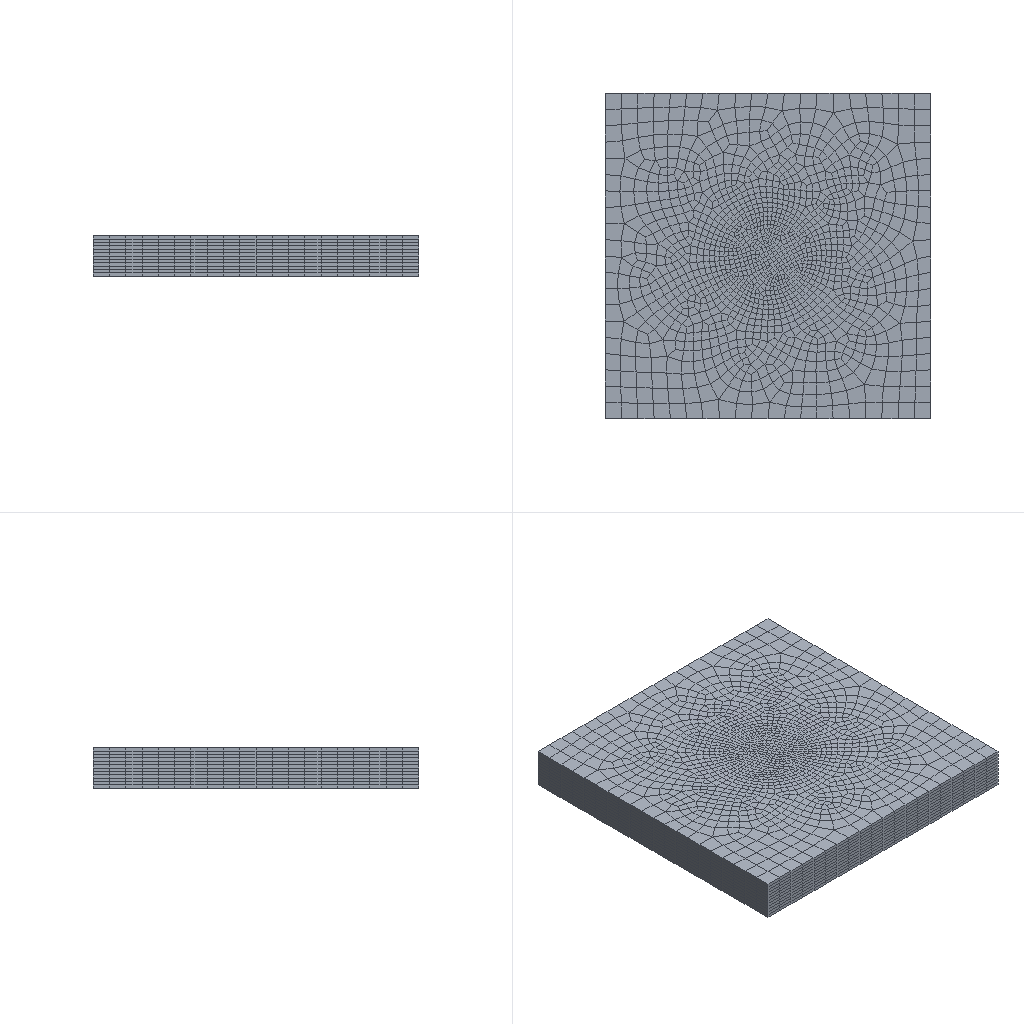Simulation study | abaqus
Set-up summary:
category,name,step,type,value,unit,region
solver,abaqus
solver,version,,,Abaqus/Explicit 3DEXPERIENCE R2017x
units,not stated in the deck,,not stated
analysis,deck,,transient,transient
load_step,Step-1,Step-1,transient
load_step,requested,,,1
mesh,nodes,,,22542
mesh,elements,,,20493
element_type,R3D3,,rigid,102
element_type,R3D4,,rigid,1623
element_type,C3D8R,,solid,18768
load,load commands in deck,,count,2
bc,support commands in deck,,count,7
material,MATERIAL-1,,in results
check,setup vs results,,match,"per instance, exact: element labels, types and connectivity; labels of the nodes the elements use; coordinates not compared"
Abaqus input file, long lists of numbers shortened:
*Heading
** Job name: Job-1 Model name: Model-1
** Generated by: Abaqus/CAE 2017
*Preprint, echo=NO, model=NO, history=NO, contact=NO
**
** PARTS
**
*Part, name=tool
*Node
      1,         -80., 0.00333,   2.
      2,         -80.,  -2., 0.01169
** (1674 more lines like these left out)
*Element, type=R3D3
1, 457, 455, 453
2,   5, 460, 388
** (100 more lines like these left out)
*Element, type=R3D4
 3, 384, 455, 448, 383
 4, 383, 448, 382,   3
** (1621 more lines like these left out)
*Node
   1677,  -116.732,           0.,           0.
*Nset, nset=tool-RefPt_, internal
1677,
*Elset, elset=tool, generate
    1,  1725,     1
*End Part
**
*Part, name=work
*Node
      1,           0.,           0.,           0.
      2,          40.,           0.,           0.
** (20863 more lines like these left out)
*Element, type=C3D8R
    1,   146,   145,   335,   339,  2406,  2405,  4797,  4801
    2,   333,   340,   143,   142,  4795,  4802,  2403,  2402
** (18766 more lines like these left out)
*Nset, nset=Set-7, generate
     1,  20865,      1
*Elset, elset=Set-7, generate
     1,  18768,      1
*Orientation, name=Ori-1
1., 0., 0., 0., 1., 0.
1, 0.
** Section: Section-1
*Solid Section, elset=Set-7, orientation=Ori-1, material=Material-1
,
*End Part
**
**
** ASSEMBLY
**
*Assembly, name=Assembly
**
*Instance, name=work-1, part=work
*End Instance
**
*Instance, name=tool-1, part=tool
    20.586,         -20.,         122.
    20.586,         -20.,         122.,     20.586,         -21.,         122.,          90.
*End Instance
**
*Nset, nset=Set-2, instance=work-1
    1,    2,    3,    4,    5,    6,   12,   13,   14,   15,   16,   17,   18,   19,   20,   21
   22,   23,   24,   25,   26,   27,   28,   29,   30,   31,   32,   33,   34,   35,   36,   37
** (72 more lines like these left out)
*Elset, elset=Set-2, instance=work-1, generate
    1,  1106,     1
*Nset, nset=Set-3, instance=tool-1
 1677,
*Nset, nset=Set-4, instance=tool-1
 1677,
*Nset, nset=s_Set-1, instance=work-1
     5,     6,    11,    88,    89,    90,    91,    92,    93,    94,    95,    96,    97,    98,    99,   100
   101,   102,   103,   104,   105,   106,   107,   108,   109,   110,   111,   112,   113,   114,   115,   116
** (397 more lines like these left out)
*Elset, elset=s_Set-1, instance=work-1, generate
 13273,  18768,      1
*Elset, elset=_m_Surf-1_SPOS, internal, instance=tool-1, generate
   33,  1725,     1
*Surface, type=ELEMENT, name=m_Surf-1
_m_Surf-1_SPOS, SPOS
*Surface, type=NODE, name=s_Set-1_CNS_, internal
s_Set-1, 1.
*Rigid Body, ref node=tool-1.tool-RefPt_, elset=tool-1.tool
*End Assembly
**
** MATERIALS
**
*Material, name=Material-1
*Density
 1.38e-09,
*Depvar, delete=1
      6,
*Elastic, type=ENGINEERING CONSTANTS
25400.,25400.,71600.,  0.35,  0.25,  0.25, 2100., 2420.
 2420.,
*User Defined Field
**
** INTERACTION PROPERTIES
**
*Surface Interaction, name=IntProp-1
*Friction
 0.2,
*Surface Behavior, pressure-overclosure=HARD
** ----------------------------------------------------------------
**
** STEP: Step-1
**
*Step, name=Step-1, nlgeom=YES
*Dynamic, Explicit
, 0.1
*Bulk Viscosity
0.06, 1.2
** Mass Scaling: Semi-Automatic
**               Whole Model
*Fixed Mass Scaling, factor=500.
**
** BOUNDARY CONDITIONS
**
** Name: BC-1 Type: 对称/反对称/完全固定
*Boundary
Set-2, ENCASTRE
** Name: BC-2 Type: 速度/角速度
*Boundary, type=VELOCITY
Set-4, 1, 1
Set-4, 2, 2
Set-4, 3, 3, -100.
Set-4, 4, 4
Set-4, 5, 5
Set-4, 6, 6, -733.
**
** INTERACTIONS
**
** Interaction: Int-1
*Contact Pair, interaction=IntProp-1, mechanical constraint=KINEMATIC, cpset=Int-1
m_Surf-1, s_Set-1_CNS_
**
** OUTPUT REQUESTS
**
*Restart, write, number interval=1, time marks=NO
**
** FIELD OUTPUT: F-Output-1
**
*Output, field, number interval=100
*Node Output
A, RF, RM, U, V
*Element Output, directions=YES
E, FV, LE, MFR, MISES, PE, PEEQ, PEEQVAVG, PEVAVG, S, SDV, STATUS, SVAVG, UVARM
*Contact Output
CSTRESS,
**
** HISTORY OUTPUT: H-Output-1
**
*Output, history, time interval=0.0001
*Node Output, nset=Set-4
RF1, RF2, RF3, RM1, RM2, RM3
*End Step
Results summary:
result,step,Step-1,completed,increments=686292 time=0.1/0.1
result,analysis,,,transient
result,last_loadstep,,,1
result,primary field,,,U
result,reaction total,,FX,-3279.888,model units
result,reaction total,,FY,-2916.926,model units
result,reaction total,,FZ,-1325.696,model units